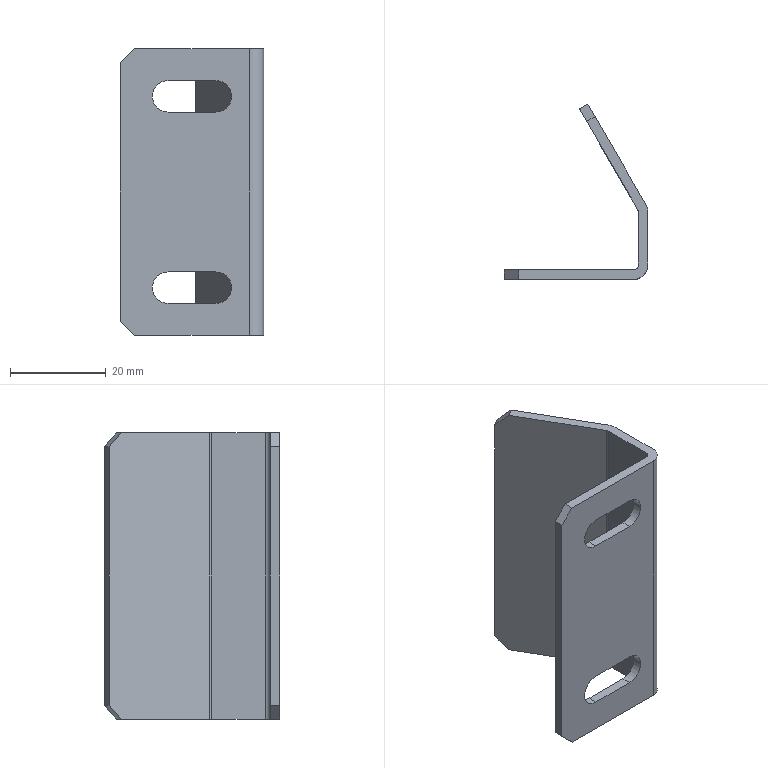Part | SolidWorks | features BaseBody 1 | 1 solid | 26 faces | box 30 x 36.651 x 60 mm | volume 7553 mm3 | plane 18 | cylinder 8 | commonest cylinder face diameters 6.6 x4 2 x2 6 x2
STEP:
#1=CARTESIAN_POINT('',(-14.232,35.651,-27.));
#2=VERTEX_POINT('',#1);
#3=CARTESIAN_POINT('',(-12.732,33.053,-30.));
#4=VERTEX_POINT('',#3);
#5=CARTESIAN_POINT('',(-22.232,49.507,-11.));
#6=DIRECTION('',(0.3536,-0.6124,-0.7071));
#7=VECTOR('',#6,1000.);
#8=LINE('',#5,#7);
#9=EDGE_CURVE('',#2,#4,#8,.T.);
#10=ORIENTED_EDGE('',*,*,#9,.F.);
#11=CARTESIAN_POINT('',(-12.5,36.651,-27.));
#12=VERTEX_POINT('',#11);
#13=CARTESIAN_POINT('',(-14.232,35.651,-27.));
#14=DIRECTION('',(-0.866,-0.5,0.));
#15=VECTOR('',#14,1000.);
#16=LINE('',#13,#15);
#17=EDGE_CURVE('',#12,#2,#16,.T.);
#18=ORIENTED_EDGE('',*,*,#17,.F.);
#19=CARTESIAN_POINT('',(-11.,34.053,-30.));
#20=VERTEX_POINT('',#19);
#21=CARTESIAN_POINT('',(-11.,34.053,-30.));
#22=DIRECTION('',(-0.3536,0.6124,0.7071));
#23=VECTOR('',#22,1000.);
#24=LINE('',#21,#23);
#25=EDGE_CURVE('',#20,#12,#24,.T.);
#26=ORIENTED_EDGE('',*,*,#25,.F.);
#27=CARTESIAN_POINT('',(-12.848,32.986,-30.));
#28=DIRECTION('',(0.866,0.5,0.));
#29=VECTOR('',#28,1000.);
#30=LINE('',#27,#29);
#31=EDGE_CURVE('',#4,#20,#30,.T.);
#32=ORIENTED_EDGE('',*,*,#31,.F.);
#33=EDGE_LOOP('',(#10,#18,#26,#32));
#34=FACE_OUTER_BOUND('',#33,.T.);
#35=CARTESIAN_POINT('',(-12.848,32.986,-30.));
#36=DIRECTION('',(0.3536,-0.6124,0.7071));
#37=DIRECTION('',(-0.866,-0.5,0.));
#38=AXIS2_PLACEMENT_3D('',#35,#36,#37);
#39=PLANE('',#38);
#40=ADVANCED_FACE('',(#34),#39,.F.);
#41=CARTESIAN_POINT('',(-30.,0.,-27.));
#42=VERTEX_POINT('',#41);
#43=CARTESIAN_POINT('',(-27.,0.,-30.));
#44=VERTEX_POINT('',#43);
#45=CARTESIAN_POINT('',(-27.,0.,-30.));
#46=DIRECTION('',(0.7071,0.,-0.7071));
#47=VECTOR('',#46,1000.);
#48=LINE('',#45,#47);
#49=EDGE_CURVE('',#42,#44,#48,.T.);
#50=ORIENTED_EDGE('',*,*,#49,.F.);
#51=CARTESIAN_POINT('',(-30.,2.,-27.));
#52=VERTEX_POINT('',#51);
#53=CARTESIAN_POINT('',(-30.,0.,-27.));
#54=DIRECTION('',(0.,-1.,0.));
#55=VECTOR('',#54,1000.);
#56=LINE('',#53,#55);
#57=EDGE_CURVE('',#52,#42,#56,.T.);
#58=ORIENTED_EDGE('',*,*,#57,.F.);
#59=CARTESIAN_POINT('',(-27.,2.,-30.));
#60=VERTEX_POINT('',#59);
#61=CARTESIAN_POINT('',(-58.5,2.,1.5));
#62=DIRECTION('',(-0.7071,0.,0.7071));
#63=VECTOR('',#62,1000.);
#64=LINE('',#61,#63);
#65=EDGE_CURVE('',#60,#52,#64,.T.);
#66=ORIENTED_EDGE('',*,*,#65,.F.);
#67=CARTESIAN_POINT('',(-27.,2.,-30.));
#68=DIRECTION('',(0.,1.,0.));
#69=VECTOR('',#68,1000.);
#70=LINE('',#67,#69);
#71=EDGE_CURVE('',#44,#60,#70,.T.);
#72=ORIENTED_EDGE('',*,*,#71,.F.);
#73=EDGE_LOOP('',(#50,#58,#66,#72));
#74=FACE_OUTER_BOUND('',#73,.T.);
#75=CARTESIAN_POINT('',(-27.,14.196,-30.));
#76=DIRECTION('',(-0.7071,0.,-0.7071));
#77=DIRECTION('',(-0.7071,0.,0.7071));
#78=AXIS2_PLACEMENT_3D('',#75,#76,#77);
#79=PLANE('',#78);
#80=ADVANCED_FACE('',(#74),#79,.T.);
#81=CARTESIAN_POINT('',(-12.732,33.053,30.));
#82=VERTEX_POINT('',#81);
#83=CARTESIAN_POINT('',(-14.232,35.651,27.));
#84=VERTEX_POINT('',#83);
#85=CARTESIAN_POINT('',(-7.232,23.526,41.));
#86=DIRECTION('',(-0.3536,0.6124,-0.7071));
#87=VECTOR('',#86,1000.);
#88=LINE('',#85,#87);
#89=EDGE_CURVE('',#82,#84,#88,.T.);
#90=ORIENTED_EDGE('',*,*,#89,.F.);
#91=CARTESIAN_POINT('',(-11.,34.053,30.));
#92=VERTEX_POINT('',#91);
#93=CARTESIAN_POINT('',(-13.598,32.553,30.));
#94=DIRECTION('',(-0.866,-0.5,0.));
#95=VECTOR('',#94,1000.);
#96=LINE('',#93,#95);
#97=EDGE_CURVE('',#92,#82,#96,.T.);
#98=ORIENTED_EDGE('',*,*,#97,.F.);
#99=CARTESIAN_POINT('',(-12.5,36.651,27.));
#100=VERTEX_POINT('',#99);
#101=CARTESIAN_POINT('',(-12.5,36.651,27.));
#102=DIRECTION('',(0.3536,-0.6124,0.7071));
#103=VECTOR('',#102,1000.);
#104=LINE('',#101,#103);
#105=EDGE_CURVE('',#100,#92,#104,.T.);
#106=ORIENTED_EDGE('',*,*,#105,.F.);
#107=CARTESIAN_POINT('',(-14.232,35.651,27.));
#108=DIRECTION('',(0.866,0.5,0.));
#109=VECTOR('',#108,1000.);
#110=LINE('',#107,#109);
#111=EDGE_CURVE('',#84,#100,#110,.T.);
#112=ORIENTED_EDGE('',*,*,#111,.F.);
#113=EDGE_LOOP('',(#90,#98,#106,#112));
#114=FACE_OUTER_BOUND('',#113,.T.);
#115=CARTESIAN_POINT('',(-14.232,35.651,27.));
#116=DIRECTION('',(0.3536,-0.6124,-0.7071));
#117=DIRECTION('',(0.,-0.7559,0.6547));
#118=AXIS2_PLACEMENT_3D('',#115,#116,#117);
#119=PLANE('',#118);
#120=ADVANCED_FACE('',(#114),#119,.F.);
#121=CARTESIAN_POINT('',(-27.,0.,30.));
#122=VERTEX_POINT('',#121);
#123=CARTESIAN_POINT('',(-30.,0.,27.));
#124=VERTEX_POINT('',#123);
#125=CARTESIAN_POINT('',(-30.,0.,27.));
#126=DIRECTION('',(-0.7071,0.,-0.7071));
#127=VECTOR('',#126,1000.);
#128=LINE('',#125,#127);
#129=EDGE_CURVE('',#122,#124,#128,.T.);
#130=ORIENTED_EDGE('',*,*,#129,.F.);
#131=CARTESIAN_POINT('',(-27.,2.,30.));
#132=VERTEX_POINT('',#131);
#133=CARTESIAN_POINT('',(-27.,3.,30.));
#134=DIRECTION('',(0.,-1.,0.));
#135=VECTOR('',#134,1000.);
#136=LINE('',#133,#135);
#137=EDGE_CURVE('',#132,#122,#136,.T.);
#138=ORIENTED_EDGE('',*,*,#137,.F.);
#139=CARTESIAN_POINT('',(-30.,2.,27.));
#140=VERTEX_POINT('',#139);
#141=CARTESIAN_POINT('',(-28.5,2.,28.5));
#142=DIRECTION('',(0.7071,0.,0.7071));
#143=VECTOR('',#142,1000.);
#144=LINE('',#141,#143);
#145=EDGE_CURVE('',#140,#132,#144,.T.);
#146=ORIENTED_EDGE('',*,*,#145,.F.);
#147=CARTESIAN_POINT('',(-30.,0.,27.));
#148=DIRECTION('',(0.,1.,0.));
#149=VECTOR('',#148,1000.);
#150=LINE('',#147,#149);
#151=EDGE_CURVE('',#124,#140,#150,.T.);
#152=ORIENTED_EDGE('',*,*,#151,.F.);
#153=EDGE_LOOP('',(#130,#138,#146,#152));
#154=FACE_OUTER_BOUND('',#153,.T.);
#155=CARTESIAN_POINT('',(-30.,0.,27.));
#156=DIRECTION('',(0.7071,0.,-0.7071));
#157=DIRECTION('',(0.,-1.,0.));
#158=AXIS2_PLACEMENT_3D('',#155,#156,#157);
#159=PLANE('',#158);
#160=ADVANCED_FACE('',(#154),#159,.F.);
#161=CARTESIAN_POINT('',(-20.,0.,23.3));
#162=VERTEX_POINT('',#161);
#163=CARTESIAN_POINT('',(-20.,2.,23.3));
#164=VERTEX_POINT('',#163);
#165=CARTESIAN_POINT('',(-20.,2.,23.3));
#166=DIRECTION('',(0.,1.,0.));
#167=VECTOR('',#166,1000.);
#168=LINE('',#165,#167);
#169=EDGE_CURVE('',#162,#164,#168,.T.);
#170=ORIENTED_EDGE('',*,*,#169,.T.);
#171=CARTESIAN_POINT('',(-10.,2.,23.3));
#172=VERTEX_POINT('',#171);
#173=CARTESIAN_POINT('',(-20.,2.,23.3));
#174=DIRECTION('',(1.,0.,0.));
#175=VECTOR('',#174,1000.);
#176=LINE('',#173,#175);
#177=EDGE_CURVE('',#164,#172,#176,.T.);
#178=ORIENTED_EDGE('',*,*,#177,.T.);
#179=CARTESIAN_POINT('',(-10.,0.,23.3));
#180=VERTEX_POINT('',#179);
#181=CARTESIAN_POINT('',(-10.,2.,23.3));
#182=DIRECTION('',(0.,-1.,0.));
#183=VECTOR('',#182,1000.);
#184=LINE('',#181,#183);
#185=EDGE_CURVE('',#172,#180,#184,.T.);
#186=ORIENTED_EDGE('',*,*,#185,.T.);
#187=CARTESIAN_POINT('',(-30.,0.,23.3));
#188=DIRECTION('',(1.,0.,0.));
#189=VECTOR('',#188,1000.);
#190=LINE('',#187,#189);
#191=EDGE_CURVE('',#162,#180,#190,.T.);
#192=ORIENTED_EDGE('',*,*,#191,.F.);
#193=EDGE_LOOP('',(#170,#178,#186,#192));
#194=FACE_OUTER_BOUND('',#193,.T.);
#195=CARTESIAN_POINT('',(-20.,2.,23.3));
#196=DIRECTION('',(0.,0.,1.));
#197=DIRECTION('',(1.,0.,0.));
#198=AXIS2_PLACEMENT_3D('',#195,#196,#197);
#199=PLANE('',#198);
#200=ADVANCED_FACE('',(#194),#199,.F.);
#201=CARTESIAN_POINT('',(-10.,0.,16.7));
#202=VERTEX_POINT('',#201);
#203=CARTESIAN_POINT('',(-10.,2.,16.7));
#204=VERTEX_POINT('',#203);
#205=CARTESIAN_POINT('',(-10.,2.,16.7));
#206=DIRECTION('',(0.,1.,0.));
#207=VECTOR('',#206,1000.);
#208=LINE('',#205,#207);
#209=EDGE_CURVE('',#202,#204,#208,.T.);
#210=ORIENTED_EDGE('',*,*,#209,.T.);
#211=CARTESIAN_POINT('',(-20.,2.,16.7));
#212=VERTEX_POINT('',#211);
#213=CARTESIAN_POINT('',(-20.,2.,16.7));
#214=DIRECTION('',(1.,0.,0.));
#215=VECTOR('',#214,1000.);
#216=LINE('',#213,#215);
#217=EDGE_CURVE('',#212,#204,#216,.T.);
#218=ORIENTED_EDGE('',*,*,#217,.F.);
#219=CARTESIAN_POINT('',(-20.,0.,16.7));
#220=VERTEX_POINT('',#219);
#221=CARTESIAN_POINT('',(-20.,2.,16.7));
#222=DIRECTION('',(0.,-1.,0.));
#223=VECTOR('',#222,1000.);
#224=LINE('',#221,#223);
#225=EDGE_CURVE('',#212,#220,#224,.T.);
#226=ORIENTED_EDGE('',*,*,#225,.T.);
#227=CARTESIAN_POINT('',(-30.,0.,16.7));
#228=DIRECTION('',(-1.,0.,0.));
#229=VECTOR('',#228,1000.);
#230=LINE('',#227,#229);
#231=EDGE_CURVE('',#202,#220,#230,.T.);
#232=ORIENTED_EDGE('',*,*,#231,.F.);
#233=EDGE_LOOP('',(#210,#218,#226,#232));
#234=FACE_OUTER_BOUND('',#233,.T.);
#235=CARTESIAN_POINT('',(-20.,2.,16.7));
#236=DIRECTION('',(0.,0.,-1.));
#237=DIRECTION('',(0.,-1.,0.));
#238=AXIS2_PLACEMENT_3D('',#235,#236,#237);
#239=PLANE('',#238);
#240=ADVANCED_FACE('',(#234),#239,.F.);
#241=ORIENTED_EDGE('',*,*,#225,.F.);
#242=CARTESIAN_POINT('',(-20.,2.,20.));
#243=DIRECTION('',(0.,1.,0.));
#244=DIRECTION('',(0.,0.,1.));
#245=AXIS2_PLACEMENT_3D('',#242,#243,#244);
#246=CIRCLE('',#245,3.3);
#247=EDGE_CURVE('',#212,#164,#246,.T.);
#248=ORIENTED_EDGE('',*,*,#247,.T.);
#249=ORIENTED_EDGE('',*,*,#169,.F.);
#250=CARTESIAN_POINT('',(-20.,0.,20.));
#251=DIRECTION('',(0.,1.,0.));
#252=DIRECTION('',(0.,0.,1.));
#253=AXIS2_PLACEMENT_3D('',#250,#251,#252);
#254=CIRCLE('',#253,3.3);
#255=EDGE_CURVE('',#220,#162,#254,.T.);
#256=ORIENTED_EDGE('',*,*,#255,.F.);
#257=EDGE_LOOP('',(#241,#248,#249,#256));
#258=FACE_OUTER_BOUND('',#257,.T.);
#259=CARTESIAN_POINT('',(-20.,2.,20.));
#260=DIRECTION('',(0.,1.,0.));
#261=DIRECTION('',(0.,0.,1.));
#262=AXIS2_PLACEMENT_3D('',#259,#260,#261);
#263=CYLINDRICAL_SURFACE('',#262,3.3);
#264=ADVANCED_FACE('',(#258),#263,.F.);
#265=ORIENTED_EDGE('',*,*,#185,.F.);
#266=CARTESIAN_POINT('',(-10.,2.,20.));
#267=DIRECTION('',(0.,1.,0.));
#268=DIRECTION('',(0.,0.,1.));
#269=AXIS2_PLACEMENT_3D('',#266,#267,#268);
#270=CIRCLE('',#269,3.3);
#271=EDGE_CURVE('',#172,#204,#270,.T.);
#272=ORIENTED_EDGE('',*,*,#271,.T.);
#273=ORIENTED_EDGE('',*,*,#209,.F.);
#274=CARTESIAN_POINT('',(-10.,0.,20.));
#275=DIRECTION('',(0.,1.,0.));
#276=DIRECTION('',(0.,0.,1.));
#277=AXIS2_PLACEMENT_3D('',#274,#275,#276);
#278=CIRCLE('',#277,3.3);
#279=EDGE_CURVE('',#180,#202,#278,.T.);
#280=ORIENTED_EDGE('',*,*,#279,.F.);
#281=EDGE_LOOP('',(#265,#272,#273,#280));
#282=FACE_OUTER_BOUND('',#281,.T.);
#283=CARTESIAN_POINT('',(-10.,2.,20.));
#284=DIRECTION('',(0.,1.,0.));
#285=DIRECTION('',(0.,0.,1.));
#286=AXIS2_PLACEMENT_3D('',#283,#284,#285);
#287=CYLINDRICAL_SURFACE('',#286,3.3);
#288=ADVANCED_FACE('',(#282),#287,.F.);
#289=CARTESIAN_POINT('',(-20.,0.,-16.7));
#290=VERTEX_POINT('',#289);
#291=CARTESIAN_POINT('',(-20.,2.,-16.7));
#292=VERTEX_POINT('',#291);
#293=CARTESIAN_POINT('',(-20.,2.,-16.7));
#294=DIRECTION('',(0.,1.,0.));
#295=VECTOR('',#294,1000.);
#296=LINE('',#293,#295);
#297=EDGE_CURVE('',#290,#292,#296,.T.);
#298=ORIENTED_EDGE('',*,*,#297,.T.);
#299=CARTESIAN_POINT('',(-10.,2.,-16.7));
#300=VERTEX_POINT('',#299);
#301=CARTESIAN_POINT('',(-20.,2.,-16.7));
#302=DIRECTION('',(1.,0.,0.));
#303=VECTOR('',#302,1000.);
#304=LINE('',#301,#303);
#305=EDGE_CURVE('',#292,#300,#304,.T.);
#306=ORIENTED_EDGE('',*,*,#305,.T.);
#307=CARTESIAN_POINT('',(-10.,0.,-16.7));
#308=VERTEX_POINT('',#307);
#309=CARTESIAN_POINT('',(-10.,2.,-16.7));
#310=DIRECTION('',(0.,-1.,0.));
#311=VECTOR('',#310,1000.);
#312=LINE('',#309,#311);
#313=EDGE_CURVE('',#300,#308,#312,.T.);
#314=ORIENTED_EDGE('',*,*,#313,.T.);
#315=CARTESIAN_POINT('',(-30.,0.,-16.7));
#316=DIRECTION('',(1.,0.,0.));
#317=VECTOR('',#316,1000.);
#318=LINE('',#315,#317);
#319=EDGE_CURVE('',#290,#308,#318,.T.);
#320=ORIENTED_EDGE('',*,*,#319,.F.);
#321=EDGE_LOOP('',(#298,#306,#314,#320));
#322=FACE_OUTER_BOUND('',#321,.T.);
#323=CARTESIAN_POINT('',(-20.,2.,-16.7));
#324=DIRECTION('',(0.,0.,1.));
#325=DIRECTION('',(1.,0.,0.));
#326=AXIS2_PLACEMENT_3D('',#323,#324,#325);
#327=PLANE('',#326);
#328=ADVANCED_FACE('',(#322),#327,.F.);
#329=CARTESIAN_POINT('',(-10.,0.,-23.3));
#330=VERTEX_POINT('',#329);
#331=CARTESIAN_POINT('',(-10.,2.,-23.3));
#332=VERTEX_POINT('',#331);
#333=CARTESIAN_POINT('',(-10.,2.,-23.3));
#334=DIRECTION('',(0.,1.,0.));
#335=VECTOR('',#334,1000.);
#336=LINE('',#333,#335);
#337=EDGE_CURVE('',#330,#332,#336,.T.);
#338=ORIENTED_EDGE('',*,*,#337,.T.);
#339=CARTESIAN_POINT('',(-20.,2.,-23.3));
#340=VERTEX_POINT('',#339);
#341=CARTESIAN_POINT('',(-20.,2.,-23.3));
#342=DIRECTION('',(1.,0.,0.));
#343=VECTOR('',#342,1000.);
#344=LINE('',#341,#343);
#345=EDGE_CURVE('',#340,#332,#344,.T.);
#346=ORIENTED_EDGE('',*,*,#345,.F.);
#347=CARTESIAN_POINT('',(-20.,0.,-23.3));
#348=VERTEX_POINT('',#347);
#349=CARTESIAN_POINT('',(-20.,2.,-23.3));
#350=DIRECTION('',(0.,-1.,0.));
#351=VECTOR('',#350,1000.);
#352=LINE('',#349,#351);
#353=EDGE_CURVE('',#340,#348,#352,.T.);
#354=ORIENTED_EDGE('',*,*,#353,.T.);
#355=CARTESIAN_POINT('',(-30.,0.,-23.3));
#356=DIRECTION('',(-1.,0.,0.));
#357=VECTOR('',#356,1000.);
#358=LINE('',#355,#357);
#359=EDGE_CURVE('',#330,#348,#358,.T.);
#360=ORIENTED_EDGE('',*,*,#359,.F.);
#361=EDGE_LOOP('',(#338,#346,#354,#360));
#362=FACE_OUTER_BOUND('',#361,.T.);
#363=CARTESIAN_POINT('',(-20.,2.,-23.3));
#364=DIRECTION('',(0.,0.,-1.));
#365=DIRECTION('',(0.,-1.,0.));
#366=AXIS2_PLACEMENT_3D('',#363,#364,#365);
#367=PLANE('',#366);
#368=ADVANCED_FACE('',(#362),#367,.F.);
#369=ORIENTED_EDGE('',*,*,#353,.F.);
#370=CARTESIAN_POINT('',(-20.,2.,-20.));
#371=DIRECTION('',(0.,1.,0.));
#372=DIRECTION('',(0.,0.,1.));
#373=AXIS2_PLACEMENT_3D('',#370,#371,#372);
#374=CIRCLE('',#373,3.3);
#375=EDGE_CURVE('',#340,#292,#374,.T.);
#376=ORIENTED_EDGE('',*,*,#375,.T.);
#377=ORIENTED_EDGE('',*,*,#297,.F.);
#378=CARTESIAN_POINT('',(-20.,0.,-20.));
#379=DIRECTION('',(0.,1.,0.));
#380=DIRECTION('',(0.,0.,1.));
#381=AXIS2_PLACEMENT_3D('',#378,#379,#380);
#382=CIRCLE('',#381,3.3);
#383=EDGE_CURVE('',#348,#290,#382,.T.);
#384=ORIENTED_EDGE('',*,*,#383,.F.);
#385=EDGE_LOOP('',(#369,#376,#377,#384));
#386=FACE_OUTER_BOUND('',#385,.T.);
#387=CARTESIAN_POINT('',(-20.,2.,-20.));
#388=DIRECTION('',(0.,1.,0.));
#389=DIRECTION('',(0.,0.,1.));
#390=AXIS2_PLACEMENT_3D('',#387,#388,#389);
#391=CYLINDRICAL_SURFACE('',#390,3.3);
#392=ADVANCED_FACE('',(#386),#391,.F.);
#393=ORIENTED_EDGE('',*,*,#313,.F.);
#394=CARTESIAN_POINT('',(-10.,2.,-20.));
#395=DIRECTION('',(0.,1.,0.));
#396=DIRECTION('',(0.,0.,1.));
#397=AXIS2_PLACEMENT_3D('',#394,#395,#396);
#398=CIRCLE('',#397,3.3);
#399=EDGE_CURVE('',#300,#332,#398,.T.);
#400=ORIENTED_EDGE('',*,*,#399,.T.);
#401=ORIENTED_EDGE('',*,*,#337,.F.);
#402=CARTESIAN_POINT('',(-10.,0.,-20.));
#403=DIRECTION('',(0.,1.,0.));
#404=DIRECTION('',(0.,0.,1.));
#405=AXIS2_PLACEMENT_3D('',#402,#403,#404);
#406=CIRCLE('',#405,3.3);
#407=EDGE_CURVE('',#308,#330,#406,.T.);
#408=ORIENTED_EDGE('',*,*,#407,.F.);
#409=EDGE_LOOP('',(#393,#400,#401,#408));
#410=FACE_OUTER_BOUND('',#409,.T.);
#411=CARTESIAN_POINT('',(-10.,2.,-20.));
#412=DIRECTION('',(0.,1.,0.));
#413=DIRECTION('',(0.,0.,1.));
#414=AXIS2_PLACEMENT_3D('',#411,#412,#413);
#415=CYLINDRICAL_SURFACE('',#414,3.3);
#416=ADVANCED_FACE('',(#410),#415,.F.);
#417=CARTESIAN_POINT('',(0.,14.196,-30.));
#418=VERTEX_POINT('',#417);
#419=CARTESIAN_POINT('',(-0.4019,15.696,-30.));
#420=VERTEX_POINT('',#419);
#421=CARTESIAN_POINT('',(-3.,14.196,-30.));
#422=DIRECTION('',(0.,0.,1.));
#423=DIRECTION('',(-1.,0.,0.));
#424=AXIS2_PLACEMENT_3D('',#421,#422,#423);
#425=CIRCLE('',#424,3.);
#426=EDGE_CURVE('',#418,#420,#425,.T.);
#427=ORIENTED_EDGE('',*,*,#426,.T.);
#428=CARTESIAN_POINT('',(-0.4019,15.696,30.));
#429=VERTEX_POINT('',#428);
#430=CARTESIAN_POINT('',(-0.4019,15.696,30.));
#431=DIRECTION('',(0.,0.,-1.));
#432=VECTOR('',#431,1000.);
#433=LINE('',#430,#432);
#434=EDGE_CURVE('',#429,#420,#433,.T.);
#435=ORIENTED_EDGE('',*,*,#434,.F.);
#436=CARTESIAN_POINT('',(0.,14.196,30.));
#437=VERTEX_POINT('',#436);
#438=CARTESIAN_POINT('',(-3.,14.196,30.));
#439=DIRECTION('',(0.,0.,1.));
#440=DIRECTION('',(-1.,0.,0.));
#441=AXIS2_PLACEMENT_3D('',#438,#439,#440);
#442=CIRCLE('',#441,3.);
#443=EDGE_CURVE('',#437,#429,#442,.T.);
#444=ORIENTED_EDGE('',*,*,#443,.F.);
#445=CARTESIAN_POINT('',(0.,14.196,30.));
#446=DIRECTION('',(0.,0.,-1.));
#447=VECTOR('',#446,1000.);
#448=LINE('',#445,#447);
#449=EDGE_CURVE('',#437,#418,#448,.T.);
#450=ORIENTED_EDGE('',*,*,#449,.T.);
#451=EDGE_LOOP('',(#427,#435,#444,#450));
#452=FACE_OUTER_BOUND('',#451,.T.);
#453=CARTESIAN_POINT('',(-3.,14.196,30.));
#454=DIRECTION('',(0.,0.,-1.));
#455=DIRECTION('',(-1.,0.,0.));
#456=AXIS2_PLACEMENT_3D('',#453,#454,#455);
#457=CYLINDRICAL_SURFACE('',#456,3.);
#458=ADVANCED_FACE('',(#452),#457,.T.);
#459=CARTESIAN_POINT('',(0.,3.,-30.));
#460=VERTEX_POINT('',#459);
#461=CARTESIAN_POINT('',(0.,0.,-30.));
#462=DIRECTION('',(0.,1.,0.));
#463=VECTOR('',#462,1000.);
#464=LINE('',#461,#463);
#465=EDGE_CURVE('',#460,#418,#464,.T.);
#466=ORIENTED_EDGE('',*,*,#465,.T.);
#467=ORIENTED_EDGE('',*,*,#449,.F.);
#468=CARTESIAN_POINT('',(0.,3.,30.));
#469=VERTEX_POINT('',#468);
#470=CARTESIAN_POINT('',(0.,0.,30.));
#471=DIRECTION('',(0.,1.,0.));
#472=VECTOR('',#471,1000.);
#473=LINE('',#470,#472);
#474=EDGE_CURVE('',#469,#437,#473,.T.);
#475=ORIENTED_EDGE('',*,*,#474,.F.);
#476=CARTESIAN_POINT('',(0.,3.,30.));
#477=DIRECTION('',(0.,0.,-1.));
#478=VECTOR('',#477,1000.);
#479=LINE('',#476,#478);
#480=EDGE_CURVE('',#469,#460,#479,.T.);
#481=ORIENTED_EDGE('',*,*,#480,.T.);
#482=EDGE_LOOP('',(#466,#467,#475,#481));
#483=FACE_OUTER_BOUND('',#482,.T.);
#484=CARTESIAN_POINT('',(0.,0.,30.));
#485=DIRECTION('',(-1.,0.,0.));
#486=DIRECTION('',(0.,0.,1.));
#487=AXIS2_PLACEMENT_3D('',#484,#485,#486);
#488=PLANE('',#487);
#489=ADVANCED_FACE('',(#483),#488,.F.);
#490=CARTESIAN_POINT('',(-3.,0.,-30.));
#491=VERTEX_POINT('',#490);
#492=CARTESIAN_POINT('',(-3.,3.,-30.));
#493=DIRECTION('',(0.,0.,1.));
#494=DIRECTION('',(-1.,0.,0.));
#495=AXIS2_PLACEMENT_3D('',#492,#493,#494);
#496=CIRCLE('',#495,3.);
#497=EDGE_CURVE('',#491,#460,#496,.T.);
#498=ORIENTED_EDGE('',*,*,#497,.T.);
#499=ORIENTED_EDGE('',*,*,#480,.F.);
#500=CARTESIAN_POINT('',(-3.,0.,30.));
#501=VERTEX_POINT('',#500);
#502=CARTESIAN_POINT('',(-3.,3.,30.));
#503=DIRECTION('',(0.,0.,1.));
#504=DIRECTION('',(-1.,0.,0.));
#505=AXIS2_PLACEMENT_3D('',#502,#503,#504);
#506=CIRCLE('',#505,3.);
#507=EDGE_CURVE('',#501,#469,#506,.T.);
#508=ORIENTED_EDGE('',*,*,#507,.F.);
#509=CARTESIAN_POINT('',(-3.,0.,30.));
#510=DIRECTION('',(0.,0.,-1.));
#511=VECTOR('',#510,1000.);
#512=LINE('',#509,#511);
#513=EDGE_CURVE('',#501,#491,#512,.T.);
#514=ORIENTED_EDGE('',*,*,#513,.T.);
#515=EDGE_LOOP('',(#498,#499,#508,#514));
#516=FACE_OUTER_BOUND('',#515,.T.);
#517=CARTESIAN_POINT('',(-3.,3.,30.));
#518=DIRECTION('',(0.,0.,-1.));
#519=DIRECTION('',(-1.,0.,0.));
#520=AXIS2_PLACEMENT_3D('',#517,#518,#519);
#521=CYLINDRICAL_SURFACE('',#520,3.);
#522=ADVANCED_FACE('',(#516),#521,.T.);
#523=ORIENTED_EDGE('',*,*,#407,.T.);
#524=ORIENTED_EDGE('',*,*,#359,.T.);
#525=ORIENTED_EDGE('',*,*,#383,.T.);
#526=ORIENTED_EDGE('',*,*,#319,.T.);
#527=EDGE_LOOP('',(#523,#524,#525,#526));
#528=FACE_BOUND('',#527,.T.);
#529=ORIENTED_EDGE('',*,*,#279,.T.);
#530=ORIENTED_EDGE('',*,*,#231,.T.);
#531=ORIENTED_EDGE('',*,*,#255,.T.);
#532=ORIENTED_EDGE('',*,*,#191,.T.);
#533=EDGE_LOOP('',(#529,#530,#531,#532));
#534=FACE_BOUND('',#533,.T.);
#535=CARTESIAN_POINT('',(-30.,0.,30.));
#536=DIRECTION('',(1.,0.,0.));
#537=VECTOR('',#536,1000.);
#538=LINE('',#535,#537);
#539=EDGE_CURVE('',#122,#501,#538,.T.);
#540=ORIENTED_EDGE('',*,*,#539,.F.);
#541=ORIENTED_EDGE('',*,*,#129,.T.);
#542=CARTESIAN_POINT('',(-30.,0.,30.));
#543=DIRECTION('',(0.,0.,-1.));
#544=VECTOR('',#543,1000.);
#545=LINE('',#542,#544);
#546=EDGE_CURVE('',#124,#42,#545,.T.);
#547=ORIENTED_EDGE('',*,*,#546,.T.);
#548=ORIENTED_EDGE('',*,*,#49,.T.);
#549=CARTESIAN_POINT('',(-30.,0.,-30.));
#550=DIRECTION('',(1.,0.,0.));
#551=VECTOR('',#550,1000.);
#552=LINE('',#549,#551);
#553=EDGE_CURVE('',#44,#491,#552,.T.);
#554=ORIENTED_EDGE('',*,*,#553,.T.);
#555=ORIENTED_EDGE('',*,*,#513,.F.);
#556=EDGE_LOOP('',(#540,#541,#547,#548,#554,#555));
#557=FACE_OUTER_BOUND('',#556,.T.);
#558=CARTESIAN_POINT('',(-30.,0.,30.));
#559=DIRECTION('',(0.,1.,0.));
#560=DIRECTION('',(1.,0.,0.));
#561=AXIS2_PLACEMENT_3D('',#558,#559,#560);
#562=PLANE('',#561);
#563=ADVANCED_FACE('',(#528,#534,#557),#562,.F.);
#564=ORIENTED_EDGE('',*,*,#546,.F.);
#565=ORIENTED_EDGE('',*,*,#151,.T.);
#566=CARTESIAN_POINT('',(-30.,2.,30.));
#567=DIRECTION('',(0.,0.,-1.));
#568=VECTOR('',#567,1000.);
#569=LINE('',#566,#568);
#570=EDGE_CURVE('',#140,#52,#569,.T.);
#571=ORIENTED_EDGE('',*,*,#570,.T.);
#572=ORIENTED_EDGE('',*,*,#57,.T.);
#573=EDGE_LOOP('',(#564,#565,#571,#572));
#574=FACE_OUTER_BOUND('',#573,.T.);
#575=CARTESIAN_POINT('',(-30.,0.,30.));
#576=DIRECTION('',(-1.,0.,0.));
#577=DIRECTION('',(0.,0.,1.));
#578=AXIS2_PLACEMENT_3D('',#575,#576,#577);
#579=PLANE('',#578);
#580=ADVANCED_FACE('',(#574),#579,.T.);
#581=ORIENTED_EDGE('',*,*,#399,.F.);
#582=ORIENTED_EDGE('',*,*,#305,.F.);
#583=ORIENTED_EDGE('',*,*,#375,.F.);
#584=ORIENTED_EDGE('',*,*,#345,.T.);
#585=EDGE_LOOP('',(#581,#582,#583,#584));
#586=FACE_BOUND('',#585,.T.);
#587=ORIENTED_EDGE('',*,*,#177,.F.);
#588=ORIENTED_EDGE('',*,*,#247,.F.);
#589=ORIENTED_EDGE('',*,*,#217,.T.);
#590=ORIENTED_EDGE('',*,*,#271,.F.);
#591=EDGE_LOOP('',(#587,#588,#589,#590));
#592=FACE_BOUND('',#591,.T.);
#593=ORIENTED_EDGE('',*,*,#570,.F.);
#594=ORIENTED_EDGE('',*,*,#145,.T.);
#595=CARTESIAN_POINT('',(-3.,2.,30.));
#596=VERTEX_POINT('',#595);
#597=CARTESIAN_POINT('',(-30.,2.,30.));
#598=DIRECTION('',(1.,0.,0.));
#599=VECTOR('',#598,1000.);
#600=LINE('',#597,#599);
#601=EDGE_CURVE('',#132,#596,#600,.T.);
#602=ORIENTED_EDGE('',*,*,#601,.T.);
#603=CARTESIAN_POINT('',(-3.,2.,-30.));
#604=VERTEX_POINT('',#603);
#605=CARTESIAN_POINT('',(-3.,2.,30.));
#606=DIRECTION('',(0.,0.,-1.));
#607=VECTOR('',#606,1000.);
#608=LINE('',#605,#607);
#609=EDGE_CURVE('',#596,#604,#608,.T.);
#610=ORIENTED_EDGE('',*,*,#609,.T.);
#611=CARTESIAN_POINT('',(-30.,2.,-30.));
#612=DIRECTION('',(1.,0.,0.));
#613=VECTOR('',#612,1000.);
#614=LINE('',#611,#613);
#615=EDGE_CURVE('',#60,#604,#614,.T.);
#616=ORIENTED_EDGE('',*,*,#615,.F.);
#617=ORIENTED_EDGE('',*,*,#65,.T.);
#618=EDGE_LOOP('',(#593,#594,#602,#610,#616,#617));
#619=FACE_OUTER_BOUND('',#618,.T.);
#620=CARTESIAN_POINT('',(-30.,2.,30.));
#621=DIRECTION('',(0.,1.,0.));
#622=DIRECTION('',(1.,0.,0.));
#623=AXIS2_PLACEMENT_3D('',#620,#621,#622);
#624=PLANE('',#623);
#625=ADVANCED_FACE('',(#586,#592,#619),#624,.T.);
#626=CARTESIAN_POINT('',(-2.,3.,-30.));
#627=VERTEX_POINT('',#626);
#628=CARTESIAN_POINT('',(-3.,3.,-30.));
#629=DIRECTION('',(0.,0.,1.));
#630=DIRECTION('',(1.,0.,0.));
#631=AXIS2_PLACEMENT_3D('',#628,#629,#630);
#632=CIRCLE('',#631,1.);
#633=EDGE_CURVE('',#604,#627,#632,.T.);
#634=ORIENTED_EDGE('',*,*,#633,.F.);
#635=ORIENTED_EDGE('',*,*,#609,.F.);
#636=CARTESIAN_POINT('',(-2.,3.,30.));
#637=VERTEX_POINT('',#636);
#638=CARTESIAN_POINT('',(-3.,3.,30.));
#639=DIRECTION('',(0.,0.,1.));
#640=DIRECTION('',(1.,0.,0.));
#641=AXIS2_PLACEMENT_3D('',#638,#639,#640);
#642=CIRCLE('',#641,1.);
#643=EDGE_CURVE('',#596,#637,#642,.T.);
#644=ORIENTED_EDGE('',*,*,#643,.T.);
#645=CARTESIAN_POINT('',(-2.,3.,30.));
#646=DIRECTION('',(0.,0.,-1.));
#647=VECTOR('',#646,1000.);
#648=LINE('',#645,#647);
#649=EDGE_CURVE('',#637,#627,#648,.T.);
#650=ORIENTED_EDGE('',*,*,#649,.T.);
#651=EDGE_LOOP('',(#634,#635,#644,#650));
#652=FACE_OUTER_BOUND('',#651,.T.);
#653=CARTESIAN_POINT('',(-3.,3.,30.));
#654=DIRECTION('',(0.,0.,-1.));
#655=DIRECTION('',(-1.,0.,0.));
#656=AXIS2_PLACEMENT_3D('',#653,#654,#655);
#657=CYLINDRICAL_SURFACE('',#656,1.);
#658=ADVANCED_FACE('',(#652),#657,.F.);
#659=CARTESIAN_POINT('',(-2.,14.196,-30.));
#660=VERTEX_POINT('',#659);
#661=CARTESIAN_POINT('',(-2.,0.,-30.));
#662=DIRECTION('',(0.,1.,0.));
#663=VECTOR('',#662,1000.);
#664=LINE('',#661,#663);
#665=EDGE_CURVE('',#627,#660,#664,.T.);
#666=ORIENTED_EDGE('',*,*,#665,.F.);
#667=ORIENTED_EDGE('',*,*,#649,.F.);
#668=CARTESIAN_POINT('',(-2.,14.196,30.));
#669=VERTEX_POINT('',#668);
#670=CARTESIAN_POINT('',(-2.,0.,30.));
#671=DIRECTION('',(0.,1.,0.));
#672=VECTOR('',#671,1000.);
#673=LINE('',#670,#672);
#674=EDGE_CURVE('',#637,#669,#673,.T.);
#675=ORIENTED_EDGE('',*,*,#674,.T.);
#676=CARTESIAN_POINT('',(-2.,14.196,30.));
#677=DIRECTION('',(0.,0.,-1.));
#678=VECTOR('',#677,1000.);
#679=LINE('',#676,#678);
#680=EDGE_CURVE('',#669,#660,#679,.T.);
#681=ORIENTED_EDGE('',*,*,#680,.T.);
#682=EDGE_LOOP('',(#666,#667,#675,#681));
#683=FACE_OUTER_BOUND('',#682,.T.);
#684=CARTESIAN_POINT('',(-2.,0.,30.));
#685=DIRECTION('',(-1.,0.,0.));
#686=DIRECTION('',(0.,0.,1.));
#687=AXIS2_PLACEMENT_3D('',#684,#685,#686);
#688=PLANE('',#687);
#689=ADVANCED_FACE('',(#683),#688,.T.);
#690=CARTESIAN_POINT('',(-2.134,14.696,-30.));
#691=VERTEX_POINT('',#690);
#692=CARTESIAN_POINT('',(-3.,14.196,-30.));
#693=DIRECTION('',(0.,0.,1.));
#694=DIRECTION('',(1.,0.,0.));
#695=AXIS2_PLACEMENT_3D('',#692,#693,#694);
#696=CIRCLE('',#695,1.);
#697=EDGE_CURVE('',#660,#691,#696,.T.);
#698=ORIENTED_EDGE('',*,*,#697,.F.);
#699=ORIENTED_EDGE('',*,*,#680,.F.);
#700=CARTESIAN_POINT('',(-2.134,14.696,30.));
#701=VERTEX_POINT('',#700);
#702=CARTESIAN_POINT('',(-3.,14.196,30.));
#703=DIRECTION('',(0.,0.,1.));
#704=DIRECTION('',(1.,0.,0.));
#705=AXIS2_PLACEMENT_3D('',#702,#703,#704);
#706=CIRCLE('',#705,1.);
#707=EDGE_CURVE('',#669,#701,#706,.T.);
#708=ORIENTED_EDGE('',*,*,#707,.T.);
#709=CARTESIAN_POINT('',(-2.134,14.696,30.));
#710=DIRECTION('',(0.,0.,-1.));
#711=VECTOR('',#710,1000.);
#712=LINE('',#709,#711);
#713=EDGE_CURVE('',#701,#691,#712,.T.);
#714=ORIENTED_EDGE('',*,*,#713,.T.);
#715=EDGE_LOOP('',(#698,#699,#708,#714));
#716=FACE_OUTER_BOUND('',#715,.T.);
#717=CARTESIAN_POINT('',(-3.,14.196,30.));
#718=DIRECTION('',(0.,0.,-1.));
#719=DIRECTION('',(-1.,0.,0.));
#720=AXIS2_PLACEMENT_3D('',#717,#718,#719);
#721=CYLINDRICAL_SURFACE('',#720,1.);
#722=ADVANCED_FACE('',(#716),#721,.F.);
#723=CARTESIAN_POINT('',(-1.732,14.,30.));
#724=DIRECTION('',(-0.5,0.866,0.));
#725=VECTOR('',#724,1000.);
#726=LINE('',#723,#725);
#727=EDGE_CURVE('',#701,#82,#726,.T.);
#728=ORIENTED_EDGE('',*,*,#727,.T.);
#729=ORIENTED_EDGE('',*,*,#89,.T.);
#730=CARTESIAN_POINT('',(-14.232,35.651,30.));
#731=DIRECTION('',(0.,0.,-1.));
#732=VECTOR('',#731,1000.);
#733=LINE('',#730,#732);
#734=EDGE_CURVE('',#84,#2,#733,.T.);
#735=ORIENTED_EDGE('',*,*,#734,.T.);
#736=ORIENTED_EDGE('',*,*,#9,.T.);
#737=CARTESIAN_POINT('',(-1.732,14.,-30.));
#738=DIRECTION('',(-0.5,0.866,0.));
#739=VECTOR('',#738,1000.);
#740=LINE('',#737,#739);
#741=EDGE_CURVE('',#691,#4,#740,.T.);
#742=ORIENTED_EDGE('',*,*,#741,.F.);
#743=ORIENTED_EDGE('',*,*,#713,.F.);
#744=EDGE_LOOP('',(#728,#729,#735,#736,#742,#743));
#745=FACE_OUTER_BOUND('',#744,.T.);
#746=CARTESIAN_POINT('',(-1.732,14.,30.));
#747=DIRECTION('',(-0.866,-0.5,0.));
#748=DIRECTION('',(-0.5,0.866,0.));
#749=AXIS2_PLACEMENT_3D('',#746,#747,#748);
#750=PLANE('',#749);
#751=ADVANCED_FACE('',(#745),#750,.T.);
#752=ORIENTED_EDGE('',*,*,#734,.F.);
#753=ORIENTED_EDGE('',*,*,#111,.T.);
#754=CARTESIAN_POINT('',(-12.5,36.651,30.));
#755=DIRECTION('',(0.,0.,-1.));
#756=VECTOR('',#755,1000.);
#757=LINE('',#754,#756);
#758=EDGE_CURVE('',#100,#12,#757,.T.);
#759=ORIENTED_EDGE('',*,*,#758,.T.);
#760=ORIENTED_EDGE('',*,*,#17,.T.);
#761=EDGE_LOOP('',(#752,#753,#759,#760));
#762=FACE_OUTER_BOUND('',#761,.T.);
#763=CARTESIAN_POINT('',(-14.232,35.651,30.));
#764=DIRECTION('',(-0.5,0.866,0.));
#765=DIRECTION('',(0.,0.,1.));
#766=AXIS2_PLACEMENT_3D('',#763,#764,#765);
#767=PLANE('',#766);
#768=ADVANCED_FACE('',(#762),#767,.T.);
#769=ORIENTED_EDGE('',*,*,#758,.F.);
#770=ORIENTED_EDGE('',*,*,#105,.T.);
#771=CARTESIAN_POINT('',(0.,15.,30.));
#772=DIRECTION('',(-0.5,0.866,0.));
#773=VECTOR('',#772,1000.);
#774=LINE('',#771,#773);
#775=EDGE_CURVE('',#429,#92,#774,.T.);
#776=ORIENTED_EDGE('',*,*,#775,.F.);
#777=ORIENTED_EDGE('',*,*,#434,.T.);
#778=CARTESIAN_POINT('',(0.,15.,-30.));
#779=DIRECTION('',(-0.5,0.866,0.));
#780=VECTOR('',#779,1000.);
#781=LINE('',#778,#780);
#782=EDGE_CURVE('',#420,#20,#781,.T.);
#783=ORIENTED_EDGE('',*,*,#782,.T.);
#784=ORIENTED_EDGE('',*,*,#25,.T.);
#785=EDGE_LOOP('',(#769,#770,#776,#777,#783,#784));
#786=FACE_OUTER_BOUND('',#785,.T.);
#787=CARTESIAN_POINT('',(0.,15.,30.));
#788=DIRECTION('',(-0.866,-0.5,0.));
#789=DIRECTION('',(-0.5,0.866,0.));
#790=AXIS2_PLACEMENT_3D('',#787,#788,#789);
#791=PLANE('',#790);
#792=ADVANCED_FACE('',(#786),#791,.F.);
#793=ORIENTED_EDGE('',*,*,#633,.T.);
#794=ORIENTED_EDGE('',*,*,#665,.T.);
#795=ORIENTED_EDGE('',*,*,#697,.T.);
#796=ORIENTED_EDGE('',*,*,#741,.T.);
#797=ORIENTED_EDGE('',*,*,#31,.T.);
#798=ORIENTED_EDGE('',*,*,#782,.F.);
#799=ORIENTED_EDGE('',*,*,#426,.F.);
#800=ORIENTED_EDGE('',*,*,#465,.F.);
#801=ORIENTED_EDGE('',*,*,#497,.F.);
#802=ORIENTED_EDGE('',*,*,#553,.F.);
#803=ORIENTED_EDGE('',*,*,#71,.T.);
#804=ORIENTED_EDGE('',*,*,#615,.T.);
#805=EDGE_LOOP('',(#793,#794,#795,#796,#797,#798,#799,#800,#801,#802,#803,#804));
#806=FACE_OUTER_BOUND('',#805,.T.);
#807=CARTESIAN_POINT('',(0.,3.,-30.));
#808=DIRECTION('',(0.,0.,-1.));
#809=DIRECTION('',(0.,-1.,0.));
#810=AXIS2_PLACEMENT_3D('',#807,#808,#809);
#811=PLANE('',#810);
#812=ADVANCED_FACE('',(#806),#811,.T.);
#813=ORIENTED_EDGE('',*,*,#643,.F.);
#814=ORIENTED_EDGE('',*,*,#601,.F.);
#815=ORIENTED_EDGE('',*,*,#137,.T.);
#816=ORIENTED_EDGE('',*,*,#539,.T.);
#817=ORIENTED_EDGE('',*,*,#507,.T.);
#818=ORIENTED_EDGE('',*,*,#474,.T.);
#819=ORIENTED_EDGE('',*,*,#443,.T.);
#820=ORIENTED_EDGE('',*,*,#775,.T.);
#821=ORIENTED_EDGE('',*,*,#97,.T.);
#822=ORIENTED_EDGE('',*,*,#727,.F.);
#823=ORIENTED_EDGE('',*,*,#707,.F.);
#824=ORIENTED_EDGE('',*,*,#674,.F.);
#825=EDGE_LOOP('',(#813,#814,#815,#816,#817,#818,#819,#820,#821,#822,#823,#824));
#826=FACE_OUTER_BOUND('',#825,.T.);
#827=CARTESIAN_POINT('',(-3.,0.,30.));
#828=DIRECTION('',(0.,0.,1.));
#829=DIRECTION('',(1.,0.,0.));
#830=AXIS2_PLACEMENT_3D('',#827,#828,#829);
#831=PLANE('',#830);
#832=ADVANCED_FACE('',(#826),#831,.T.);
#833=CLOSED_SHELL('',(#40,#80,#120,#160,#200,#240,#264,#288,#328,#368,#392,#416,#458,#489,#522,#563,#580,#625,#658,#689,#722,#751,#768,#792,#812,#832));
#834=MANIFOLD_SOLID_BREP('',#833);
#835=CARTESIAN_POINT('',(0.,0.,0.));
#836=DIRECTION('',(0.,0.,1.));
#837=DIRECTION('',(1.,0.,0.));
#838=AXIS2_PLACEMENT_3D('',#835,#836,#837);
#839=(LENGTH_UNIT()NAMED_UNIT(*)SI_UNIT(.MILLI.,.METRE.));
#840=UNCERTAINTY_MEASURE_WITH_UNIT(LENGTH_MEASURE(0.00001),#839,'','');
#841=(NAMED_UNIT(*)PLANE_ANGLE_UNIT()SI_UNIT($,.RADIAN.));
#842=(NAMED_UNIT(*)SI_UNIT($,.STERADIAN.)SOLID_ANGLE_UNIT());
#843=(GEOMETRIC_REPRESENTATION_CONTEXT(3)GLOBAL_UNCERTAINTY_ASSIGNED_CONTEXT((#840))GLOBAL_UNIT_ASSIGNED_CONTEXT((#839,#841,#842))REPRESENTATION_CONTEXT('',''));
#844=ADVANCED_BREP_SHAPE_REPRESENTATION('',(#834,#838),#843);